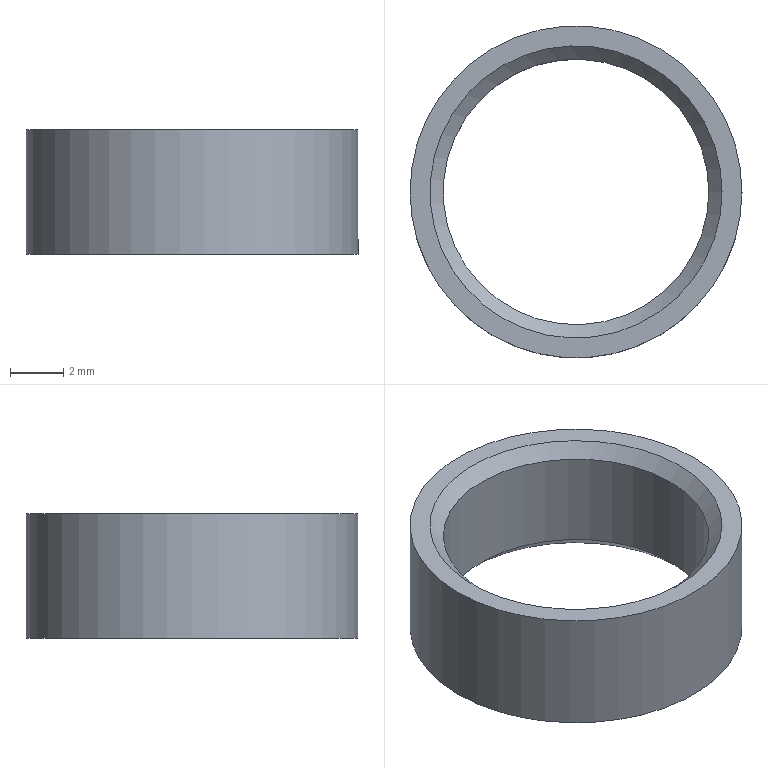Part | NX | features BREP 1 | 1 solid | 6 faces | box 12.5 x 12.5 x 4.7 mm | volume 199.524 mm3 | cone 2 | cylinder 2 | plane 2 | commonest cylinder face diameters 10 x1 12.5 x1
STEP:
#1=CARTESIAN_POINT('',(5.5,0.,0.));
#2=VERTEX_POINT('',#1);
#3=CARTESIAN_POINT('',(0.,0.,0.));
#4=DIRECTION('',(0.,0.,1.));
#5=DIRECTION('',(1.,0.,0.));
#6=AXIS2_PLACEMENT_3D('',#3,#4,#5);
#7=CIRCLE('',#6,5.5);
#8=EDGE_CURVE('',#2,#2,#7,.T.);
#9=ORIENTED_EDGE('',*,*,#8,.F.);
#10=EDGE_LOOP('',(#9));
#11=FACE_BOUND('',#10,.T.);
#12=CARTESIAN_POINT('',(5.,0.,0.5));
#13=VERTEX_POINT('',#12);
#14=CARTESIAN_POINT('',(0.,0.,0.5));
#15=DIRECTION('',(0.,0.,-1.));
#16=DIRECTION('',(1.,0.,0.));
#17=AXIS2_PLACEMENT_3D('',#14,#15,#16);
#18=CIRCLE('',#17,5.);
#19=EDGE_CURVE('',#13,#13,#18,.T.);
#20=ORIENTED_EDGE('',*,*,#19,.F.);
#21=EDGE_LOOP('',(#20));
#22=FACE_BOUND('',#21,.T.);
#23=CARTESIAN_POINT('',(0.,0.,0.));
#24=DIRECTION('',(0.,0.,-1.));
#25=DIRECTION('',(-1.,0.,0.));
#26=AXIS2_PLACEMENT_3D('',#23,#24,#25);
#27=CONICAL_SURFACE('',#26,5.5,0.7854);
#28=ADVANCED_FACE('',(#11,#22),#27,.F.);
#29=CARTESIAN_POINT('',(5.5,0.,4.7));
#30=VERTEX_POINT('',#29);
#31=CARTESIAN_POINT('',(0.,0.,4.7));
#32=DIRECTION('',(0.,0.,-1.));
#33=DIRECTION('',(1.,0.,0.));
#34=AXIS2_PLACEMENT_3D('',#31,#32,#33);
#35=CIRCLE('',#34,5.5);
#36=EDGE_CURVE('',#30,#30,#35,.T.);
#37=ORIENTED_EDGE('',*,*,#36,.F.);
#38=EDGE_LOOP('',(#37));
#39=FACE_BOUND('',#38,.T.);
#40=CARTESIAN_POINT('',(5.,0.,4.2));
#41=VERTEX_POINT('',#40);
#42=CARTESIAN_POINT('',(0.,0.,4.2));
#43=DIRECTION('',(0.,0.,1.));
#44=DIRECTION('',(1.,0.,0.));
#45=AXIS2_PLACEMENT_3D('',#42,#43,#44);
#46=CIRCLE('',#45,5.);
#47=EDGE_CURVE('',#41,#41,#46,.T.);
#48=ORIENTED_EDGE('',*,*,#47,.F.);
#49=EDGE_LOOP('',(#48));
#50=FACE_BOUND('',#49,.T.);
#51=CARTESIAN_POINT('',(0.,0.,4.2));
#52=DIRECTION('',(0.,0.,1.));
#53=DIRECTION('',(1.,0.,0.));
#54=AXIS2_PLACEMENT_3D('',#51,#52,#53);
#55=CONICAL_SURFACE('',#54,5.,0.7854);
#56=ADVANCED_FACE('',(#39,#50),#55,.F.);
#57=ORIENTED_EDGE('',*,*,#19,.T.);
#58=EDGE_LOOP('',(#57));
#59=FACE_BOUND('',#58,.T.);
#60=ORIENTED_EDGE('',*,*,#47,.T.);
#61=EDGE_LOOP('',(#60));
#62=FACE_BOUND('',#61,.T.);
#63=CARTESIAN_POINT('',(0.,0.,4.7));
#64=DIRECTION('',(0.,0.,-1.));
#65=DIRECTION('',(-1.,0.,0.));
#66=AXIS2_PLACEMENT_3D('',#63,#64,#65);
#67=CYLINDRICAL_SURFACE('',#66,5.);
#68=ADVANCED_FACE('',(#59,#62),#67,.F.);
#69=CARTESIAN_POINT('',(6.25,0.,0.));
#70=VERTEX_POINT('',#69);
#71=CARTESIAN_POINT('',(0.,0.,0.));
#72=DIRECTION('',(0.,0.,1.));
#73=DIRECTION('',(1.,0.,0.));
#74=AXIS2_PLACEMENT_3D('',#71,#72,#73);
#75=CIRCLE('',#74,6.25);
#76=EDGE_CURVE('',#70,#70,#75,.T.);
#77=ORIENTED_EDGE('',*,*,#76,.T.);
#78=EDGE_LOOP('',(#77));
#79=FACE_BOUND('',#78,.T.);
#80=CARTESIAN_POINT('',(6.25,0.,4.7));
#81=VERTEX_POINT('',#80);
#82=CARTESIAN_POINT('',(0.,0.,4.7));
#83=DIRECTION('',(0.,0.,1.));
#84=DIRECTION('',(1.,0.,0.));
#85=AXIS2_PLACEMENT_3D('',#82,#83,#84);
#86=CIRCLE('',#85,6.25);
#87=EDGE_CURVE('',#81,#81,#86,.T.);
#88=ORIENTED_EDGE('',*,*,#87,.F.);
#89=EDGE_LOOP('',(#88));
#90=FACE_BOUND('',#89,.T.);
#91=CARTESIAN_POINT('',(0.,0.,4.7));
#92=DIRECTION('',(0.,0.,-1.));
#93=DIRECTION('',(-1.,0.,0.));
#94=AXIS2_PLACEMENT_3D('',#91,#92,#93);
#95=CYLINDRICAL_SURFACE('',#94,6.25);
#96=ADVANCED_FACE('',(#79,#90),#95,.T.);
#97=ORIENTED_EDGE('',*,*,#36,.T.);
#98=EDGE_LOOP('',(#97));
#99=FACE_BOUND('',#98,.T.);
#100=ORIENTED_EDGE('',*,*,#87,.T.);
#101=EDGE_LOOP('',(#100));
#102=FACE_BOUND('',#101,.T.);
#103=CARTESIAN_POINT('',(0.,0.,4.7));
#104=DIRECTION('',(0.,0.,1.));
#105=DIRECTION('',(1.,0.,0.));
#106=AXIS2_PLACEMENT_3D('',#103,#104,#105);
#107=PLANE('',#106);
#108=ADVANCED_FACE('',(#99,#102),#107,.T.);
#109=ORIENTED_EDGE('',*,*,#8,.T.);
#110=EDGE_LOOP('',(#109));
#111=FACE_BOUND('',#110,.T.);
#112=ORIENTED_EDGE('',*,*,#76,.F.);
#113=EDGE_LOOP('',(#112));
#114=FACE_BOUND('',#113,.T.);
#115=CARTESIAN_POINT('',(0.,0.,0.));
#116=DIRECTION('',(0.,0.,1.));
#117=DIRECTION('',(1.,0.,0.));
#118=AXIS2_PLACEMENT_3D('',#115,#116,#117);
#119=PLANE('',#118);
#120=ADVANCED_FACE('',(#111,#114),#119,.F.);
#121=CLOSED_SHELL('',(#28,#56,#68,#96,#108,#120));
#122=MANIFOLD_SOLID_BREP('',#121);
#123=(LENGTH_UNIT()NAMED_UNIT(*)SI_UNIT(.MILLI.,.METRE.));
#124=UNCERTAINTY_MEASURE_WITH_UNIT(LENGTH_MEASURE(0.00001),#123,'','');
#125=(NAMED_UNIT(*)PLANE_ANGLE_UNIT()SI_UNIT($,.RADIAN.));
#126=(NAMED_UNIT(*)SI_UNIT($,.STERADIAN.)SOLID_ANGLE_UNIT());
#127=(GEOMETRIC_REPRESENTATION_CONTEXT(3)GLOBAL_UNCERTAINTY_ASSIGNED_CONTEXT((#124))GLOBAL_UNIT_ASSIGNED_CONTEXT((#123,#125,#126))REPRESENTATION_CONTEXT('',''));
#128=ADVANCED_BREP_SHAPE_REPRESENTATION('',(#122),#127);